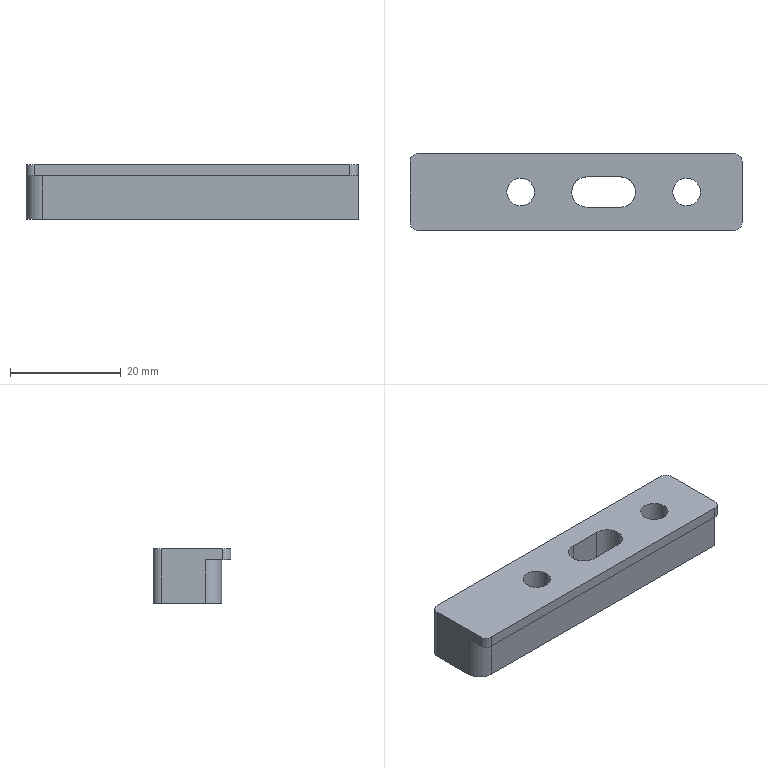Part | STEP file | 200 mesh_id10_xmt | 1 solid | 19 faces | box 60 x 14 x 9.8 mm | volume 6516 mm3 | plane 10 | cylinder 9 | commonest cylinder face diameters 3 x4 5 x2 5.5 x2 6 x1
STEP:
#1=CARTESIAN_POINT('',(-17037.648,-3977.669,50.7));
#2=VERTEX_POINT('',#1);
#3=CARTESIAN_POINT('',(-17037.648,-3977.669,42.9));
#4=VERTEX_POINT('',#3);
#5=CARTESIAN_POINT('',(-17037.648,-3977.669,50.7));
#6=DIRECTION('',(0.,0.,-1.));
#7=VECTOR('',#6,1.);
#8=LINE('',#5,#7);
#9=EDGE_CURVE('',#2,#4,#8,.T.);
#10=ORIENTED_EDGE('',*,*,#9,.T.);
#11=CARTESIAN_POINT('',(-17037.648,-3966.769,42.9));
#12=VERTEX_POINT('',#11);
#13=CARTESIAN_POINT('',(-17037.648,-3977.769,42.9));
#14=DIRECTION('',(0.,1.,0.));
#15=VECTOR('',#14,1.);
#16=LINE('',#13,#15);
#17=EDGE_CURVE('',#4,#12,#16,.T.);
#18=ORIENTED_EDGE('',*,*,#17,.T.);
#19=CARTESIAN_POINT('',(-17037.648,-3966.769,52.7));
#20=VERTEX_POINT('',#19);
#21=CARTESIAN_POINT('',(-17037.648,-3966.769,52.7));
#22=DIRECTION('',(0.,0.,-1.));
#23=VECTOR('',#22,1.);
#24=LINE('',#21,#23);
#25=EDGE_CURVE('',#20,#12,#24,.T.);
#26=ORIENTED_EDGE('',*,*,#25,.F.);
#27=CARTESIAN_POINT('',(-17037.648,-3977.769,52.7));
#28=VERTEX_POINT('',#27);
#29=CARTESIAN_POINT('',(-17037.648,-3977.769,52.7));
#30=DIRECTION('',(0.,1.,0.));
#31=VECTOR('',#30,1.);
#32=LINE('',#29,#31);
#33=EDGE_CURVE('',#28,#20,#32,.T.);
#34=ORIENTED_EDGE('',*,*,#33,.F.);
#35=CARTESIAN_POINT('',(-17037.648,-3977.769,50.7));
#36=VERTEX_POINT('',#35);
#37=CARTESIAN_POINT('',(-17037.648,-3977.769,52.7));
#38=DIRECTION('',(0.,0.,-1.));
#39=VECTOR('',#38,1.);
#40=LINE('',#37,#39);
#41=EDGE_CURVE('',#28,#36,#40,.T.);
#42=ORIENTED_EDGE('',*,*,#41,.T.);
#43=CARTESIAN_POINT('',(-17037.648,-3979.269,50.7));
#44=DIRECTION('',(0.,1.,0.));
#45=VECTOR('',#44,1.);
#46=LINE('',#43,#45);
#47=EDGE_CURVE('',#36,#2,#46,.T.);
#48=ORIENTED_EDGE('',*,*,#47,.T.);
#49=EDGE_LOOP('',(#10,#18,#26,#34,#42,#48));
#50=FACE_OUTER_BOUND('',#49,.T.);
#51=CARTESIAN_POINT('',(-17037.648,-3977.769,52.7));
#52=DIRECTION('',(-1.,0.,0.));
#53=DIRECTION('',(0.,0.,1.));
#54=AXIS2_PLACEMENT_3D('',#51,#52,#53);
#55=PLANE('',#54);
#56=ADVANCED_FACE('',(#50),#55,.F.);
#57=ORIENTED_EDGE('',*,*,#25,.T.);
#58=CARTESIAN_POINT('',(-17039.148,-3965.269,42.9));
#59=VERTEX_POINT('',#58);
#60=CARTESIAN_POINT('',(-17039.148,-3966.769,42.9));
#61=DIRECTION('',(0.,0.,1.));
#62=DIRECTION('',(1.,0.,0.));
#63=AXIS2_PLACEMENT_3D('',#60,#61,#62);
#64=CIRCLE('',#63,1.5);
#65=EDGE_CURVE('',#12,#59,#64,.T.);
#66=ORIENTED_EDGE('',*,*,#65,.T.);
#67=CARTESIAN_POINT('',(-17039.148,-3965.269,52.7));
#68=VERTEX_POINT('',#67);
#69=CARTESIAN_POINT('',(-17039.148,-3965.269,52.7));
#70=DIRECTION('',(0.,0.,-1.));
#71=VECTOR('',#70,1.);
#72=LINE('',#69,#71);
#73=EDGE_CURVE('',#68,#59,#72,.T.);
#74=ORIENTED_EDGE('',*,*,#73,.F.);
#75=CARTESIAN_POINT('',(-17039.148,-3966.769,52.7));
#76=DIRECTION('',(0.,0.,1.));
#77=DIRECTION('',(1.,0.,0.));
#78=AXIS2_PLACEMENT_3D('',#75,#76,#77);
#79=CIRCLE('',#78,1.5);
#80=EDGE_CURVE('',#20,#68,#79,.T.);
#81=ORIENTED_EDGE('',*,*,#80,.F.);
#82=EDGE_LOOP('',(#57,#66,#74,#81));
#83=FACE_OUTER_BOUND('',#82,.T.);
#84=CARTESIAN_POINT('',(-17039.148,-3966.769,52.7));
#85=DIRECTION('',(0.,0.,-1.));
#86=DIRECTION('',(-1.,0.,0.));
#87=AXIS2_PLACEMENT_3D('',#84,#85,#86);
#88=CYLINDRICAL_SURFACE('',#87,1.5);
#89=ADVANCED_FACE('',(#83),#88,.T.);
#90=ORIENTED_EDGE('',*,*,#73,.T.);
#91=CARTESIAN_POINT('',(-17096.148,-3965.269,42.9));
#92=VERTEX_POINT('',#91);
#93=CARTESIAN_POINT('',(-17039.148,-3965.269,42.9));
#94=DIRECTION('',(-1.,0.,0.));
#95=VECTOR('',#94,1.);
#96=LINE('',#93,#95);
#97=EDGE_CURVE('',#59,#92,#96,.T.);
#98=ORIENTED_EDGE('',*,*,#97,.T.);
#99=CARTESIAN_POINT('',(-17096.148,-3965.269,52.7));
#100=VERTEX_POINT('',#99);
#101=CARTESIAN_POINT('',(-17096.148,-3965.269,52.7));
#102=DIRECTION('',(0.,0.,-1.));
#103=VECTOR('',#102,1.);
#104=LINE('',#101,#103);
#105=EDGE_CURVE('',#100,#92,#104,.T.);
#106=ORIENTED_EDGE('',*,*,#105,.F.);
#107=CARTESIAN_POINT('',(-17039.148,-3965.269,52.7));
#108=DIRECTION('',(-1.,0.,0.));
#109=VECTOR('',#108,1.);
#110=LINE('',#107,#109);
#111=EDGE_CURVE('',#68,#100,#110,.T.);
#112=ORIENTED_EDGE('',*,*,#111,.F.);
#113=EDGE_LOOP('',(#90,#98,#106,#112));
#114=FACE_OUTER_BOUND('',#113,.T.);
#115=CARTESIAN_POINT('',(-17039.148,-3965.269,52.7));
#116=DIRECTION('',(0.,-1.,0.));
#117=DIRECTION('',(0.,0.,-1.));
#118=AXIS2_PLACEMENT_3D('',#115,#116,#117);
#119=PLANE('',#118);
#120=ADVANCED_FACE('',(#114),#119,.F.);
#121=CARTESIAN_POINT('',(-17097.648,-3966.769,42.9));
#122=VERTEX_POINT('',#121);
#123=CARTESIAN_POINT('',(-17096.148,-3966.769,42.9));
#124=DIRECTION('',(0.,0.,1.));
#125=DIRECTION('',(1.,0.,0.));
#126=AXIS2_PLACEMENT_3D('',#123,#124,#125);
#127=CIRCLE('',#126,1.5);
#128=EDGE_CURVE('',#92,#122,#127,.T.);
#129=ORIENTED_EDGE('',*,*,#128,.T.);
#130=CARTESIAN_POINT('',(-17097.648,-3966.769,52.7));
#131=VERTEX_POINT('',#130);
#132=CARTESIAN_POINT('',(-17097.648,-3966.769,52.7));
#133=DIRECTION('',(0.,0.,-1.));
#134=VECTOR('',#133,1.);
#135=LINE('',#132,#134);
#136=EDGE_CURVE('',#131,#122,#135,.T.);
#137=ORIENTED_EDGE('',*,*,#136,.F.);
#138=CARTESIAN_POINT('',(-17096.148,-3966.769,52.7));
#139=DIRECTION('',(0.,0.,1.));
#140=DIRECTION('',(1.,0.,0.));
#141=AXIS2_PLACEMENT_3D('',#138,#139,#140);
#142=CIRCLE('',#141,1.5);
#143=EDGE_CURVE('',#100,#131,#142,.T.);
#144=ORIENTED_EDGE('',*,*,#143,.F.);
#145=ORIENTED_EDGE('',*,*,#105,.T.);
#146=EDGE_LOOP('',(#129,#137,#144,#145));
#147=FACE_OUTER_BOUND('',#146,.T.);
#148=CARTESIAN_POINT('',(-17096.148,-3966.769,52.7));
#149=DIRECTION('',(0.,0.,-1.));
#150=DIRECTION('',(-1.,0.,0.));
#151=AXIS2_PLACEMENT_3D('',#148,#149,#150);
#152=CYLINDRICAL_SURFACE('',#151,1.5);
#153=ADVANCED_FACE('',(#147),#152,.T.);
#154=CARTESIAN_POINT('',(-17097.648,-3974.669,42.9));
#155=VERTEX_POINT('',#154);
#156=CARTESIAN_POINT('',(-17097.648,-3968.769,42.9));
#157=DIRECTION('',(0.,-1.,0.));
#158=VECTOR('',#157,1.);
#159=LINE('',#156,#158);
#160=EDGE_CURVE('',#122,#155,#159,.T.);
#161=ORIENTED_EDGE('',*,*,#160,.T.);
#162=CARTESIAN_POINT('',(-17097.648,-3974.669,50.7));
#163=VERTEX_POINT('',#162);
#164=CARTESIAN_POINT('',(-17097.648,-3974.669,52.7));
#165=DIRECTION('',(0.,0.,1.));
#166=VECTOR('',#165,1.);
#167=LINE('',#164,#166);
#168=EDGE_CURVE('',#155,#163,#167,.T.);
#169=ORIENTED_EDGE('',*,*,#168,.T.);
#170=CARTESIAN_POINT('',(-17097.648,-3977.769,50.7));
#171=VERTEX_POINT('',#170);
#172=CARTESIAN_POINT('',(-17097.648,-3968.769,50.7));
#173=DIRECTION('',(0.,-1.,0.));
#174=VECTOR('',#173,1.);
#175=LINE('',#172,#174);
#176=EDGE_CURVE('',#163,#171,#175,.T.);
#177=ORIENTED_EDGE('',*,*,#176,.T.);
#178=CARTESIAN_POINT('',(-17097.648,-3977.769,52.7));
#179=VERTEX_POINT('',#178);
#180=CARTESIAN_POINT('',(-17097.648,-3977.769,52.7));
#181=DIRECTION('',(0.,0.,-1.));
#182=VECTOR('',#181,1.);
#183=LINE('',#180,#182);
#184=EDGE_CURVE('',#179,#171,#183,.T.);
#185=ORIENTED_EDGE('',*,*,#184,.F.);
#186=CARTESIAN_POINT('',(-17097.648,-3968.769,52.7));
#187=DIRECTION('',(0.,-1.,0.));
#188=VECTOR('',#187,1.);
#189=LINE('',#186,#188);
#190=EDGE_CURVE('',#131,#179,#189,.T.);
#191=ORIENTED_EDGE('',*,*,#190,.F.);
#192=ORIENTED_EDGE('',*,*,#136,.T.);
#193=EDGE_LOOP('',(#161,#169,#177,#185,#191,#192));
#194=FACE_OUTER_BOUND('',#193,.T.);
#195=CARTESIAN_POINT('',(-17097.648,-3968.769,52.7));
#196=DIRECTION('',(1.,0.,0.));
#197=DIRECTION('',(0.,0.,-1.));
#198=AXIS2_PLACEMENT_3D('',#195,#196,#197);
#199=PLANE('',#198);
#200=ADVANCED_FACE('',(#194),#199,.F.);
#201=ORIENTED_EDGE('',*,*,#184,.T.);
#202=CARTESIAN_POINT('',(-17096.148,-3979.269,50.7));
#203=VERTEX_POINT('',#202);
#204=CARTESIAN_POINT('',(-17096.148,-3977.769,50.7));
#205=DIRECTION('',(0.,0.,1.));
#206=DIRECTION('',(1.,0.,0.));
#207=AXIS2_PLACEMENT_3D('',#204,#205,#206);
#208=CIRCLE('',#207,1.5);
#209=EDGE_CURVE('',#171,#203,#208,.T.);
#210=ORIENTED_EDGE('',*,*,#209,.T.);
#211=CARTESIAN_POINT('',(-17096.148,-3979.269,52.7));
#212=VERTEX_POINT('',#211);
#213=CARTESIAN_POINT('',(-17096.148,-3979.269,52.7));
#214=DIRECTION('',(0.,0.,-1.));
#215=VECTOR('',#214,1.);
#216=LINE('',#213,#215);
#217=EDGE_CURVE('',#212,#203,#216,.T.);
#218=ORIENTED_EDGE('',*,*,#217,.F.);
#219=CARTESIAN_POINT('',(-17096.148,-3977.769,52.7));
#220=DIRECTION('',(0.,0.,1.));
#221=DIRECTION('',(1.,0.,0.));
#222=AXIS2_PLACEMENT_3D('',#219,#220,#221);
#223=CIRCLE('',#222,1.5);
#224=EDGE_CURVE('',#179,#212,#223,.T.);
#225=ORIENTED_EDGE('',*,*,#224,.F.);
#226=EDGE_LOOP('',(#201,#210,#218,#225));
#227=FACE_OUTER_BOUND('',#226,.T.);
#228=CARTESIAN_POINT('',(-17096.148,-3977.769,52.7));
#229=DIRECTION('',(0.,0.,-1.));
#230=DIRECTION('',(-1.,0.,0.));
#231=AXIS2_PLACEMENT_3D('',#228,#229,#230);
#232=CYLINDRICAL_SURFACE('',#231,1.5);
#233=ADVANCED_FACE('',(#227),#232,.T.);
#234=ORIENTED_EDGE('',*,*,#217,.T.);
#235=CARTESIAN_POINT('',(-17039.148,-3979.269,50.7));
#236=VERTEX_POINT('',#235);
#237=CARTESIAN_POINT('',(-17037.648,-3979.269,50.7));
#238=DIRECTION('',(1.,0.,0.));
#239=VECTOR('',#238,1.);
#240=LINE('',#237,#239);
#241=EDGE_CURVE('',#203,#236,#240,.T.);
#242=ORIENTED_EDGE('',*,*,#241,.T.);
#243=CARTESIAN_POINT('',(-17039.148,-3979.269,52.7));
#244=VERTEX_POINT('',#243);
#245=CARTESIAN_POINT('',(-17039.148,-3979.269,52.7));
#246=DIRECTION('',(0.,0.,-1.));
#247=VECTOR('',#246,1.);
#248=LINE('',#245,#247);
#249=EDGE_CURVE('',#244,#236,#248,.T.);
#250=ORIENTED_EDGE('',*,*,#249,.F.);
#251=CARTESIAN_POINT('',(-17116.148,-3979.269,52.7));
#252=DIRECTION('',(1.,0.,0.));
#253=VECTOR('',#252,1.);
#254=LINE('',#251,#253);
#255=EDGE_CURVE('',#212,#244,#254,.T.);
#256=ORIENTED_EDGE('',*,*,#255,.F.);
#257=EDGE_LOOP('',(#234,#242,#250,#256));
#258=FACE_OUTER_BOUND('',#257,.T.);
#259=CARTESIAN_POINT('',(-17116.148,-3979.269,52.7));
#260=DIRECTION('',(0.,1.,0.));
#261=DIRECTION('',(0.,0.,1.));
#262=AXIS2_PLACEMENT_3D('',#259,#260,#261);
#263=PLANE('',#262);
#264=ADVANCED_FACE('',(#258),#263,.F.);
#265=ORIENTED_EDGE('',*,*,#249,.T.);
#266=CARTESIAN_POINT('',(-17039.148,-3977.769,50.7));
#267=DIRECTION('',(0.,0.,1.));
#268=DIRECTION('',(1.,0.,0.));
#269=AXIS2_PLACEMENT_3D('',#266,#267,#268);
#270=CIRCLE('',#269,1.5);
#271=EDGE_CURVE('',#236,#36,#270,.T.);
#272=ORIENTED_EDGE('',*,*,#271,.T.);
#273=ORIENTED_EDGE('',*,*,#41,.F.);
#274=CARTESIAN_POINT('',(-17039.148,-3977.769,52.7));
#275=DIRECTION('',(0.,0.,1.));
#276=DIRECTION('',(1.,0.,0.));
#277=AXIS2_PLACEMENT_3D('',#274,#275,#276);
#278=CIRCLE('',#277,1.5);
#279=EDGE_CURVE('',#244,#28,#278,.T.);
#280=ORIENTED_EDGE('',*,*,#279,.F.);
#281=EDGE_LOOP('',(#265,#272,#273,#280));
#282=FACE_OUTER_BOUND('',#281,.T.);
#283=CARTESIAN_POINT('',(-17039.148,-3977.769,52.7));
#284=DIRECTION('',(0.,0.,-1.));
#285=DIRECTION('',(-1.,0.,0.));
#286=AXIS2_PLACEMENT_3D('',#283,#284,#285);
#287=CYLINDRICAL_SURFACE('',#286,1.5);
#288=ADVANCED_FACE('',(#282),#287,.T.);
#289=CARTESIAN_POINT('',(-17065.648,-3975.019,52.7));
#290=VERTEX_POINT('',#289);
#291=CARTESIAN_POINT('',(-17059.648,-3975.019,52.7));
#292=VERTEX_POINT('',#291);
#293=CARTESIAN_POINT('',(-17062.648,-3975.019,52.7));
#294=DIRECTION('',(1.,0.,0.));
#295=VECTOR('',#294,1.);
#296=LINE('',#293,#295);
#297=EDGE_CURVE('',#290,#292,#296,.T.);
#298=ORIENTED_EDGE('',*,*,#297,.F.);
#299=CARTESIAN_POINT('',(-17065.648,-3969.519,52.7));
#300=VERTEX_POINT('',#299);
#301=CARTESIAN_POINT('',(-17065.648,-3972.269,52.7));
#302=DIRECTION('',(0.,0.,1.));
#303=DIRECTION('',(-1.,0.,0.));
#304=AXIS2_PLACEMENT_3D('',#301,#302,#303);
#305=CIRCLE('',#304,2.75);
#306=EDGE_CURVE('',#300,#290,#305,.T.);
#307=ORIENTED_EDGE('',*,*,#306,.F.);
#308=CARTESIAN_POINT('',(-17059.648,-3969.519,52.7));
#309=VERTEX_POINT('',#308);
#310=CARTESIAN_POINT('',(-17062.648,-3969.519,52.7));
#311=DIRECTION('',(-1.,0.,0.));
#312=VECTOR('',#311,1.);
#313=LINE('',#310,#312);
#314=EDGE_CURVE('',#309,#300,#313,.T.);
#315=ORIENTED_EDGE('',*,*,#314,.F.);
#316=CARTESIAN_POINT('',(-17059.648,-3972.269,52.7));
#317=DIRECTION('',(0.,0.,1.));
#318=DIRECTION('',(1.,0.,0.));
#319=AXIS2_PLACEMENT_3D('',#316,#317,#318);
#320=CIRCLE('',#319,2.75);
#321=EDGE_CURVE('',#292,#309,#320,.T.);
#322=ORIENTED_EDGE('',*,*,#321,.F.);
#323=EDGE_LOOP('',(#298,#307,#315,#322));
#324=FACE_BOUND('',#323,.T.);
#325=CARTESIAN_POINT('',(-17045.148,-3972.269,52.7));
#326=VERTEX_POINT('',#325);
#327=CARTESIAN_POINT('',(-17047.648,-3972.269,52.7));
#328=DIRECTION('',(0.,0.,1.));
#329=DIRECTION('',(1.,0.,0.));
#330=AXIS2_PLACEMENT_3D('',#327,#328,#329);
#331=CIRCLE('',#330,2.5);
#332=EDGE_CURVE('',#326,#326,#331,.T.);
#333=ORIENTED_EDGE('',*,*,#332,.F.);
#334=EDGE_LOOP('',(#333));
#335=FACE_BOUND('',#334,.T.);
#336=CARTESIAN_POINT('',(-17075.148,-3972.269,52.7));
#337=VERTEX_POINT('',#336);
#338=CARTESIAN_POINT('',(-17077.648,-3972.269,52.7));
#339=DIRECTION('',(0.,0.,1.));
#340=DIRECTION('',(1.,0.,0.));
#341=AXIS2_PLACEMENT_3D('',#338,#339,#340);
#342=CIRCLE('',#341,2.5);
#343=EDGE_CURVE('',#337,#337,#342,.T.);
#344=ORIENTED_EDGE('',*,*,#343,.F.);
#345=EDGE_LOOP('',(#344));
#346=FACE_BOUND('',#345,.T.);
#347=ORIENTED_EDGE('',*,*,#33,.T.);
#348=ORIENTED_EDGE('',*,*,#80,.T.);
#349=ORIENTED_EDGE('',*,*,#111,.T.);
#350=ORIENTED_EDGE('',*,*,#143,.T.);
#351=ORIENTED_EDGE('',*,*,#190,.T.);
#352=ORIENTED_EDGE('',*,*,#224,.T.);
#353=ORIENTED_EDGE('',*,*,#255,.T.);
#354=ORIENTED_EDGE('',*,*,#279,.T.);
#355=EDGE_LOOP('',(#347,#348,#349,#350,#351,#352,#353,#354));
#356=FACE_BOUND('',#355,.T.);
#357=CARTESIAN_POINT('',(-17039.148,-3968.769,52.7));
#358=DIRECTION('',(0.,0.,1.));
#359=DIRECTION('',(1.,0.,0.));
#360=AXIS2_PLACEMENT_3D('',#357,#358,#359);
#361=PLANE('',#360);
#362=ADVANCED_FACE('',(#324,#335,#346,#356),#361,.T.);
#363=CARTESIAN_POINT('',(-17045.148,-3972.269,42.9));
#364=VERTEX_POINT('',#363);
#365=CARTESIAN_POINT('',(-17047.648,-3972.269,42.9));
#366=DIRECTION('',(0.,0.,1.));
#367=DIRECTION('',(1.,0.,0.));
#368=AXIS2_PLACEMENT_3D('',#365,#366,#367);
#369=CIRCLE('',#368,2.5);
#370=EDGE_CURVE('',#364,#364,#369,.T.);
#371=ORIENTED_EDGE('',*,*,#370,.T.);
#372=EDGE_LOOP('',(#371));
#373=FACE_BOUND('',#372,.T.);
#374=CARTESIAN_POINT('',(-17075.148,-3972.269,42.9));
#375=VERTEX_POINT('',#374);
#376=CARTESIAN_POINT('',(-17077.648,-3972.269,42.9));
#377=DIRECTION('',(0.,0.,1.));
#378=DIRECTION('',(1.,0.,0.));
#379=AXIS2_PLACEMENT_3D('',#376,#377,#378);
#380=CIRCLE('',#379,2.5);
#381=EDGE_CURVE('',#375,#375,#380,.T.);
#382=ORIENTED_EDGE('',*,*,#381,.T.);
#383=EDGE_LOOP('',(#382));
#384=FACE_BOUND('',#383,.T.);
#385=CARTESIAN_POINT('',(-17094.648,-3977.669,42.9));
#386=VERTEX_POINT('',#385);
#387=CARTESIAN_POINT('',(-17039.148,-3977.669,42.9));
#388=DIRECTION('',(-1.,0.,0.));
#389=VECTOR('',#388,1.);
#390=LINE('',#387,#389);
#391=EDGE_CURVE('',#4,#386,#390,.T.);
#392=ORIENTED_EDGE('',*,*,#391,.T.);
#393=CARTESIAN_POINT('',(-17094.648,-3974.669,42.9));
#394=DIRECTION('',(0.,0.,-1.));
#395=DIRECTION('',(1.,0.,0.));
#396=AXIS2_PLACEMENT_3D('',#393,#394,#395);
#397=CIRCLE('',#396,3.);
#398=EDGE_CURVE('',#386,#155,#397,.T.);
#399=ORIENTED_EDGE('',*,*,#398,.T.);
#400=ORIENTED_EDGE('',*,*,#160,.F.);
#401=ORIENTED_EDGE('',*,*,#128,.F.);
#402=ORIENTED_EDGE('',*,*,#97,.F.);
#403=ORIENTED_EDGE('',*,*,#65,.F.);
#404=ORIENTED_EDGE('',*,*,#17,.F.);
#405=EDGE_LOOP('',(#392,#399,#400,#401,#402,#403,#404));
#406=FACE_BOUND('',#405,.T.);
#407=CARTESIAN_POINT('',(-17059.648,-3969.519,42.9));
#408=VERTEX_POINT('',#407);
#409=CARTESIAN_POINT('',(-17065.648,-3969.519,42.9));
#410=VERTEX_POINT('',#409);
#411=CARTESIAN_POINT('',(-17039.148,-3969.519,42.9));
#412=DIRECTION('',(-1.,0.,0.));
#413=VECTOR('',#412,1.);
#414=LINE('',#411,#413);
#415=EDGE_CURVE('',#408,#410,#414,.T.);
#416=ORIENTED_EDGE('',*,*,#415,.T.);
#417=CARTESIAN_POINT('',(-17065.648,-3975.019,42.9));
#418=VERTEX_POINT('',#417);
#419=CARTESIAN_POINT('',(-17065.648,-3972.269,42.9));
#420=DIRECTION('',(0.,0.,1.));
#421=DIRECTION('',(1.,0.,0.));
#422=AXIS2_PLACEMENT_3D('',#419,#420,#421);
#423=CIRCLE('',#422,2.75);
#424=EDGE_CURVE('',#410,#418,#423,.T.);
#425=ORIENTED_EDGE('',*,*,#424,.T.);
#426=CARTESIAN_POINT('',(-17059.648,-3975.019,42.9));
#427=VERTEX_POINT('',#426);
#428=CARTESIAN_POINT('',(-17039.148,-3975.019,42.9));
#429=DIRECTION('',(1.,0.,0.));
#430=VECTOR('',#429,1.);
#431=LINE('',#428,#430);
#432=EDGE_CURVE('',#418,#427,#431,.T.);
#433=ORIENTED_EDGE('',*,*,#432,.T.);
#434=CARTESIAN_POINT('',(-17059.648,-3972.269,42.9));
#435=DIRECTION('',(0.,0.,1.));
#436=DIRECTION('',(1.,0.,0.));
#437=AXIS2_PLACEMENT_3D('',#434,#435,#436);
#438=CIRCLE('',#437,2.75);
#439=EDGE_CURVE('',#427,#408,#438,.T.);
#440=ORIENTED_EDGE('',*,*,#439,.T.);
#441=EDGE_LOOP('',(#416,#425,#433,#440));
#442=FACE_BOUND('',#441,.T.);
#443=CARTESIAN_POINT('',(-17039.148,-3968.769,42.9));
#444=DIRECTION('',(0.,0.,1.));
#445=DIRECTION('',(1.,0.,0.));
#446=AXIS2_PLACEMENT_3D('',#443,#444,#445);
#447=PLANE('',#446);
#448=ADVANCED_FACE('',(#373,#384,#406,#442),#447,.F.);
#449=CARTESIAN_POINT('',(-17094.648,-3977.669,50.7));
#450=VERTEX_POINT('',#449);
#451=CARTESIAN_POINT('',(-17037.648,-3977.669,50.7));
#452=DIRECTION('',(1.,0.,0.));
#453=VECTOR('',#452,1.);
#454=LINE('',#451,#453);
#455=EDGE_CURVE('',#450,#2,#454,.T.);
#456=ORIENTED_EDGE('',*,*,#455,.F.);
#457=CARTESIAN_POINT('',(-17094.648,-3977.669,50.7));
#458=DIRECTION('',(0.,0.,-1.));
#459=VECTOR('',#458,1.);
#460=LINE('',#457,#459);
#461=EDGE_CURVE('',#450,#386,#460,.T.);
#462=ORIENTED_EDGE('',*,*,#461,.T.);
#463=ORIENTED_EDGE('',*,*,#391,.F.);
#464=ORIENTED_EDGE('',*,*,#9,.F.);
#465=EDGE_LOOP('',(#456,#462,#463,#464));
#466=FACE_OUTER_BOUND('',#465,.T.);
#467=CARTESIAN_POINT('',(-17037.648,-3977.669,50.7));
#468=DIRECTION('',(0.,1.,0.));
#469=DIRECTION('',(-1.,0.,0.));
#470=AXIS2_PLACEMENT_3D('',#467,#468,#469);
#471=PLANE('',#470);
#472=ADVANCED_FACE('',(#466),#471,.F.);
#473=ORIENTED_EDGE('',*,*,#176,.F.);
#474=CARTESIAN_POINT('',(-17094.648,-3974.669,50.7));
#475=DIRECTION('',(0.,0.,1.));
#476=DIRECTION('',(1.,0.,0.));
#477=AXIS2_PLACEMENT_3D('',#474,#475,#476);
#478=CIRCLE('',#477,3.);
#479=EDGE_CURVE('',#163,#450,#478,.T.);
#480=ORIENTED_EDGE('',*,*,#479,.T.);
#481=ORIENTED_EDGE('',*,*,#455,.T.);
#482=ORIENTED_EDGE('',*,*,#47,.F.);
#483=ORIENTED_EDGE('',*,*,#271,.F.);
#484=ORIENTED_EDGE('',*,*,#241,.F.);
#485=ORIENTED_EDGE('',*,*,#209,.F.);
#486=EDGE_LOOP('',(#473,#480,#481,#482,#483,#484,#485));
#487=FACE_OUTER_BOUND('',#486,.T.);
#488=CARTESIAN_POINT('',(-17037.648,-3979.269,50.7));
#489=DIRECTION('',(0.,0.,1.));
#490=DIRECTION('',(1.,0.,0.));
#491=AXIS2_PLACEMENT_3D('',#488,#489,#490);
#492=PLANE('',#491);
#493=ADVANCED_FACE('',(#487),#492,.F.);
#494=ORIENTED_EDGE('',*,*,#343,.T.);
#495=EDGE_LOOP('',(#494));
#496=FACE_BOUND('',#495,.T.);
#497=ORIENTED_EDGE('',*,*,#381,.F.);
#498=EDGE_LOOP('',(#497));
#499=FACE_BOUND('',#498,.T.);
#500=CARTESIAN_POINT('',(-17077.648,-3972.269,42.9));
#501=DIRECTION('',(0.,0.,1.));
#502=DIRECTION('',(1.,0.,0.));
#503=AXIS2_PLACEMENT_3D('',#500,#501,#502);
#504=CYLINDRICAL_SURFACE('',#503,2.5);
#505=ADVANCED_FACE('',(#496,#499),#504,.F.);
#506=ORIENTED_EDGE('',*,*,#332,.T.);
#507=EDGE_LOOP('',(#506));
#508=FACE_BOUND('',#507,.T.);
#509=ORIENTED_EDGE('',*,*,#370,.F.);
#510=EDGE_LOOP('',(#509));
#511=FACE_BOUND('',#510,.T.);
#512=CARTESIAN_POINT('',(-17047.648,-3972.269,42.9));
#513=DIRECTION('',(0.,0.,1.));
#514=DIRECTION('',(1.,0.,0.));
#515=AXIS2_PLACEMENT_3D('',#512,#513,#514);
#516=CYLINDRICAL_SURFACE('',#515,2.5);
#517=ADVANCED_FACE('',(#508,#511),#516,.F.);
#518=ORIENTED_EDGE('',*,*,#398,.F.);
#519=ORIENTED_EDGE('',*,*,#461,.F.);
#520=ORIENTED_EDGE('',*,*,#479,.F.);
#521=ORIENTED_EDGE('',*,*,#168,.F.);
#522=EDGE_LOOP('',(#518,#519,#520,#521));
#523=FACE_OUTER_BOUND('',#522,.T.);
#524=CARTESIAN_POINT('',(-17094.648,-3974.669,52.7));
#525=DIRECTION('',(0.,0.,1.));
#526=DIRECTION('',(1.,0.,0.));
#527=AXIS2_PLACEMENT_3D('',#524,#525,#526);
#528=CYLINDRICAL_SURFACE('',#527,3.);
#529=ADVANCED_FACE('',(#523),#528,.T.);
#530=CARTESIAN_POINT('',(-17065.648,-3969.519,28.2));
#531=DIRECTION('',(0.,0.,-1.));
#532=VECTOR('',#531,1.);
#533=LINE('',#530,#532);
#534=EDGE_CURVE('',#300,#410,#533,.T.);
#535=ORIENTED_EDGE('',*,*,#534,.F.);
#536=ORIENTED_EDGE('',*,*,#306,.T.);
#537=CARTESIAN_POINT('',(-17065.648,-3975.019,28.2));
#538=DIRECTION('',(0.,0.,-1.));
#539=VECTOR('',#538,1.);
#540=LINE('',#537,#539);
#541=EDGE_CURVE('',#290,#418,#540,.T.);
#542=ORIENTED_EDGE('',*,*,#541,.T.);
#543=ORIENTED_EDGE('',*,*,#424,.F.);
#544=EDGE_LOOP('',(#535,#536,#542,#543));
#545=FACE_OUTER_BOUND('',#544,.T.);
#546=CARTESIAN_POINT('',(-17065.648,-3972.269,28.2));
#547=DIRECTION('',(0.,0.,1.));
#548=DIRECTION('',(1.,0.,0.));
#549=AXIS2_PLACEMENT_3D('',#546,#547,#548);
#550=CYLINDRICAL_SURFACE('',#549,2.75);
#551=ADVANCED_FACE('',(#545),#550,.F.);
#552=ORIENTED_EDGE('',*,*,#297,.T.);
#553=CARTESIAN_POINT('',(-17059.648,-3975.019,28.2));
#554=DIRECTION('',(0.,0.,-1.));
#555=VECTOR('',#554,1.);
#556=LINE('',#553,#555);
#557=EDGE_CURVE('',#292,#427,#556,.T.);
#558=ORIENTED_EDGE('',*,*,#557,.T.);
#559=ORIENTED_EDGE('',*,*,#432,.F.);
#560=ORIENTED_EDGE('',*,*,#541,.F.);
#561=EDGE_LOOP('',(#552,#558,#559,#560));
#562=FACE_OUTER_BOUND('',#561,.T.);
#563=CARTESIAN_POINT('',(-17062.648,-3975.019,28.2));
#564=DIRECTION('',(0.,-1.,0.));
#565=DIRECTION('',(0.,0.,-1.));
#566=AXIS2_PLACEMENT_3D('',#563,#564,#565);
#567=PLANE('',#566);
#568=ADVANCED_FACE('',(#562),#567,.F.);
#569=ORIENTED_EDGE('',*,*,#557,.F.);
#570=ORIENTED_EDGE('',*,*,#321,.T.);
#571=CARTESIAN_POINT('',(-17059.648,-3969.519,28.2));
#572=DIRECTION('',(0.,0.,-1.));
#573=VECTOR('',#572,1.);
#574=LINE('',#571,#573);
#575=EDGE_CURVE('',#309,#408,#574,.T.);
#576=ORIENTED_EDGE('',*,*,#575,.T.);
#577=ORIENTED_EDGE('',*,*,#439,.F.);
#578=EDGE_LOOP('',(#569,#570,#576,#577));
#579=FACE_OUTER_BOUND('',#578,.T.);
#580=CARTESIAN_POINT('',(-17059.648,-3972.269,28.2));
#581=DIRECTION('',(0.,0.,1.));
#582=DIRECTION('',(1.,0.,0.));
#583=AXIS2_PLACEMENT_3D('',#580,#581,#582);
#584=CYLINDRICAL_SURFACE('',#583,2.75);
#585=ADVANCED_FACE('',(#579),#584,.F.);
#586=ORIENTED_EDGE('',*,*,#314,.T.);
#587=ORIENTED_EDGE('',*,*,#534,.T.);
#588=ORIENTED_EDGE('',*,*,#415,.F.);
#589=ORIENTED_EDGE('',*,*,#575,.F.);
#590=EDGE_LOOP('',(#586,#587,#588,#589));
#591=FACE_OUTER_BOUND('',#590,.T.);
#592=CARTESIAN_POINT('',(-17062.648,-3969.519,28.2));
#593=DIRECTION('',(0.,1.,0.));
#594=DIRECTION('',(0.,0.,1.));
#595=AXIS2_PLACEMENT_3D('',#592,#593,#594);
#596=PLANE('',#595);
#597=ADVANCED_FACE('',(#591),#596,.F.);
#598=CLOSED_SHELL('',(#56,#89,#120,#153,#200,#233,#264,#288,#362,#448,#472,#493,#505,#517,#529,#551,#568,#585,#597));
#599=MANIFOLD_SOLID_BREP('',#598);
#600=(LENGTH_UNIT()NAMED_UNIT(*)SI_UNIT(.MILLI.,.METRE.));
#601=UNCERTAINTY_MEASURE_WITH_UNIT(LENGTH_MEASURE(0.00002),#600,'','');
#602=(NAMED_UNIT(*)PLANE_ANGLE_UNIT()SI_UNIT($,.RADIAN.));
#603=PLANE_ANGLE_MEASURE_WITH_UNIT(PLANE_ANGLE_MEASURE(0.01745),#602);
#604=DIMENSIONAL_EXPONENTS(0.,0.,0.,0.,0.,0.,0.);
#605=(CONVERSION_BASED_UNIT('DEGREE',#603)NAMED_UNIT(#604)PLANE_ANGLE_UNIT());
#606=(NAMED_UNIT(*)SI_UNIT($,.STERADIAN.)SOLID_ANGLE_UNIT());
#607=(GEOMETRIC_REPRESENTATION_CONTEXT(3)GLOBAL_UNCERTAINTY_ASSIGNED_CONTEXT((#601))GLOBAL_UNIT_ASSIGNED_CONTEXT((#600,#605,#606))REPRESENTATION_CONTEXT('',''));
#608=ADVANCED_BREP_SHAPE_REPRESENTATION('',(#599),#607);